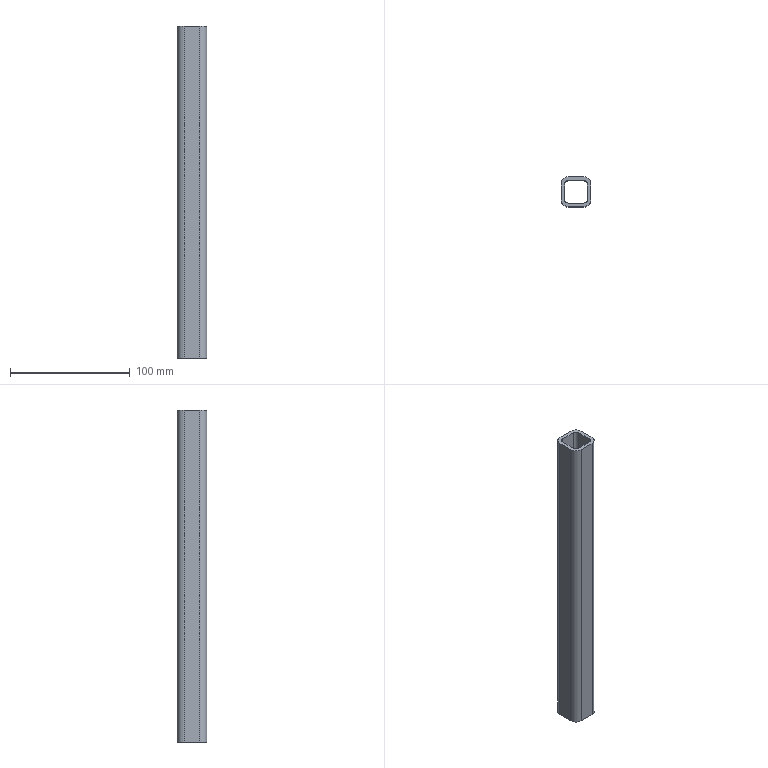Part | STEP file | ISO 10799-2 25x25x3 1784908143849 | 1 solid | 18 faces | box 25 x 25 x 277.531 mm | volume 66836 mm3 | plane 10 | cylinder 8 | commonest cylinder face diameters 6 x4 12 x4
STEP:
#1=CARTESIAN_POINT('',(-6.5,-9.5,290.031));
#2=VERTEX_POINT('',#1);
#3=CARTESIAN_POINT('',(6.5,-9.5,290.031));
#4=VERTEX_POINT('',#3);
#5=CARTESIAN_POINT('',(3.25,-9.5,290.031));
#6=DIRECTION('',(1.,0.,0.));
#7=VECTOR('',#6,10.);
#8=LINE('',#5,#7);
#9=EDGE_CURVE('',#2,#4,#8,.T.);
#10=ORIENTED_EDGE('',*,*,#9,.T.);
#11=CARTESIAN_POINT('',(6.5,-9.5,12.5));
#12=VERTEX_POINT('',#11);
#13=CARTESIAN_POINT('',(6.5,-9.5,0.));
#14=DIRECTION('',(0.,0.,1.));
#15=VECTOR('',#14,10.);
#16=LINE('',#13,#15);
#17=EDGE_CURVE('',#12,#4,#16,.T.);
#18=ORIENTED_EDGE('',*,*,#17,.F.);
#19=CARTESIAN_POINT('',(-6.5,-9.5,12.5));
#20=VERTEX_POINT('',#19);
#21=CARTESIAN_POINT('',(3.25,-9.5,12.5));
#22=DIRECTION('',(1.,0.,0.));
#23=VECTOR('',#22,10.);
#24=LINE('',#21,#23);
#25=EDGE_CURVE('',#20,#12,#24,.T.);
#26=ORIENTED_EDGE('',*,*,#25,.F.);
#27=CARTESIAN_POINT('',(-6.5,-9.5,0.));
#28=DIRECTION('',(0.,0.,1.));
#29=VECTOR('',#28,10.);
#30=LINE('',#27,#29);
#31=EDGE_CURVE('',#20,#2,#30,.T.);
#32=ORIENTED_EDGE('',*,*,#31,.T.);
#33=EDGE_LOOP('',(#10,#18,#26,#32));
#34=FACE_OUTER_BOUND('',#33,.T.);
#35=CARTESIAN_POINT('',(6.5,-9.5,0.));
#36=DIRECTION('',(0.,-1.,0.));
#37=DIRECTION('',(0.,0.,-1.));
#38=AXIS2_PLACEMENT_3D('',#35,#36,#37);
#39=PLANE('',#38);
#40=ADVANCED_FACE('',(#34),#39,.F.);
#41=CARTESIAN_POINT('',(9.5,-6.5,290.031));
#42=VERTEX_POINT('',#41);
#43=CARTESIAN_POINT('',(6.5,-6.5,290.031));
#44=DIRECTION('',(0.,0.,1.));
#45=DIRECTION('',(0.,1.,0.));
#46=AXIS2_PLACEMENT_3D('',#43,#44,#45);
#47=CIRCLE('',#46,3.);
#48=EDGE_CURVE('',#4,#42,#47,.T.);
#49=ORIENTED_EDGE('',*,*,#48,.T.);
#50=CARTESIAN_POINT('',(9.5,-6.5,12.5));
#51=VERTEX_POINT('',#50);
#52=CARTESIAN_POINT('',(9.5,-6.5,0.));
#53=DIRECTION('',(0.,0.,1.));
#54=VECTOR('',#53,10.);
#55=LINE('',#52,#54);
#56=EDGE_CURVE('',#51,#42,#55,.T.);
#57=ORIENTED_EDGE('',*,*,#56,.F.);
#58=CARTESIAN_POINT('',(6.5,-6.5,12.5));
#59=DIRECTION('',(0.,0.,1.));
#60=DIRECTION('',(0.,1.,0.));
#61=AXIS2_PLACEMENT_3D('',#58,#59,#60);
#62=CIRCLE('',#61,3.);
#63=EDGE_CURVE('',#12,#51,#62,.T.);
#64=ORIENTED_EDGE('',*,*,#63,.F.);
#65=ORIENTED_EDGE('',*,*,#17,.T.);
#66=EDGE_LOOP('',(#49,#57,#64,#65));
#67=FACE_OUTER_BOUND('',#66,.T.);
#68=CARTESIAN_POINT('',(6.5,-6.5,0.));
#69=DIRECTION('',(0.,0.,1.));
#70=DIRECTION('',(0.,1.,0.));
#71=AXIS2_PLACEMENT_3D('',#68,#69,#70);
#72=CYLINDRICAL_SURFACE('',#71,3.);
#73=ADVANCED_FACE('',(#67),#72,.F.);
#74=CARTESIAN_POINT('',(9.5,6.5,290.031));
#75=VERTEX_POINT('',#74);
#76=CARTESIAN_POINT('',(9.5,3.25,290.031));
#77=DIRECTION('',(0.,1.,0.));
#78=VECTOR('',#77,10.);
#79=LINE('',#76,#78);
#80=EDGE_CURVE('',#42,#75,#79,.T.);
#81=ORIENTED_EDGE('',*,*,#80,.T.);
#82=CARTESIAN_POINT('',(9.5,6.5,12.5));
#83=VERTEX_POINT('',#82);
#84=CARTESIAN_POINT('',(9.5,6.5,0.));
#85=DIRECTION('',(0.,0.,1.));
#86=VECTOR('',#85,10.);
#87=LINE('',#84,#86);
#88=EDGE_CURVE('',#83,#75,#87,.T.);
#89=ORIENTED_EDGE('',*,*,#88,.F.);
#90=CARTESIAN_POINT('',(9.5,3.25,12.5));
#91=DIRECTION('',(0.,1.,0.));
#92=VECTOR('',#91,10.);
#93=LINE('',#90,#92);
#94=EDGE_CURVE('',#51,#83,#93,.T.);
#95=ORIENTED_EDGE('',*,*,#94,.F.);
#96=ORIENTED_EDGE('',*,*,#56,.T.);
#97=EDGE_LOOP('',(#81,#89,#95,#96));
#98=FACE_OUTER_BOUND('',#97,.T.);
#99=CARTESIAN_POINT('',(9.5,6.5,0.));
#100=DIRECTION('',(1.,0.,0.));
#101=DIRECTION('',(0.,0.,-1.));
#102=AXIS2_PLACEMENT_3D('',#99,#100,#101);
#103=PLANE('',#102);
#104=ADVANCED_FACE('',(#98),#103,.F.);
#105=CARTESIAN_POINT('',(6.5,9.5,290.031));
#106=VERTEX_POINT('',#105);
#107=CARTESIAN_POINT('',(6.5,6.5,290.031));
#108=DIRECTION('',(0.,0.,1.));
#109=DIRECTION('',(-1.,0.,0.));
#110=AXIS2_PLACEMENT_3D('',#107,#108,#109);
#111=CIRCLE('',#110,3.);
#112=EDGE_CURVE('',#75,#106,#111,.T.);
#113=ORIENTED_EDGE('',*,*,#112,.T.);
#114=CARTESIAN_POINT('',(6.5,9.5,12.5));
#115=VERTEX_POINT('',#114);
#116=CARTESIAN_POINT('',(6.5,9.5,0.));
#117=DIRECTION('',(0.,0.,1.));
#118=VECTOR('',#117,10.);
#119=LINE('',#116,#118);
#120=EDGE_CURVE('',#115,#106,#119,.T.);
#121=ORIENTED_EDGE('',*,*,#120,.F.);
#122=CARTESIAN_POINT('',(6.5,6.5,12.5));
#123=DIRECTION('',(0.,0.,1.));
#124=DIRECTION('',(-1.,0.,0.));
#125=AXIS2_PLACEMENT_3D('',#122,#123,#124);
#126=CIRCLE('',#125,3.);
#127=EDGE_CURVE('',#83,#115,#126,.T.);
#128=ORIENTED_EDGE('',*,*,#127,.F.);
#129=ORIENTED_EDGE('',*,*,#88,.T.);
#130=EDGE_LOOP('',(#113,#121,#128,#129));
#131=FACE_OUTER_BOUND('',#130,.T.);
#132=CARTESIAN_POINT('',(6.5,6.5,0.));
#133=DIRECTION('',(0.,0.,1.));
#134=DIRECTION('',(-1.,0.,0.));
#135=AXIS2_PLACEMENT_3D('',#132,#133,#134);
#136=CYLINDRICAL_SURFACE('',#135,3.);
#137=ADVANCED_FACE('',(#131),#136,.F.);
#138=CARTESIAN_POINT('',(12.5,6.5,290.031));
#139=VERTEX_POINT('',#138);
#140=CARTESIAN_POINT('',(12.5,-6.5,290.031));
#141=VERTEX_POINT('',#140);
#142=CARTESIAN_POINT('',(12.5,3.25,290.031));
#143=DIRECTION('',(0.,-1.,0.));
#144=VECTOR('',#143,10.);
#145=LINE('',#142,#144);
#146=EDGE_CURVE('',#139,#141,#145,.T.);
#147=ORIENTED_EDGE('',*,*,#146,.T.);
#148=CARTESIAN_POINT('',(12.5,-6.5,12.5));
#149=VERTEX_POINT('',#148);
#150=CARTESIAN_POINT('',(12.5,-6.5,0.));
#151=DIRECTION('',(0.,0.,1.));
#152=VECTOR('',#151,10.);
#153=LINE('',#150,#152);
#154=EDGE_CURVE('',#149,#141,#153,.T.);
#155=ORIENTED_EDGE('',*,*,#154,.F.);
#156=CARTESIAN_POINT('',(12.5,6.5,12.5));
#157=VERTEX_POINT('',#156);
#158=CARTESIAN_POINT('',(12.5,3.25,12.5));
#159=DIRECTION('',(0.,-1.,0.));
#160=VECTOR('',#159,10.);
#161=LINE('',#158,#160);
#162=EDGE_CURVE('',#157,#149,#161,.T.);
#163=ORIENTED_EDGE('',*,*,#162,.F.);
#164=CARTESIAN_POINT('',(12.5,6.5,0.));
#165=DIRECTION('',(0.,0.,1.));
#166=VECTOR('',#165,10.);
#167=LINE('',#164,#166);
#168=EDGE_CURVE('',#157,#139,#167,.T.);
#169=ORIENTED_EDGE('',*,*,#168,.T.);
#170=EDGE_LOOP('',(#147,#155,#163,#169));
#171=FACE_OUTER_BOUND('',#170,.T.);
#172=CARTESIAN_POINT('',(12.5,6.5,0.));
#173=DIRECTION('',(1.,0.,0.));
#174=DIRECTION('',(0.,0.,-1.));
#175=AXIS2_PLACEMENT_3D('',#172,#173,#174);
#176=PLANE('',#175);
#177=ADVANCED_FACE('',(#171),#176,.T.);
#178=CARTESIAN_POINT('',(6.5,-12.5,290.031));
#179=VERTEX_POINT('',#178);
#180=CARTESIAN_POINT('',(6.5,-6.5,290.031));
#181=DIRECTION('',(0.,0.,-1.));
#182=DIRECTION('',(0.,1.,0.));
#183=AXIS2_PLACEMENT_3D('',#180,#181,#182);
#184=CIRCLE('',#183,6.);
#185=EDGE_CURVE('',#141,#179,#184,.T.);
#186=ORIENTED_EDGE('',*,*,#185,.T.);
#187=CARTESIAN_POINT('',(6.5,-12.5,12.5));
#188=VERTEX_POINT('',#187);
#189=CARTESIAN_POINT('',(6.5,-12.5,0.));
#190=DIRECTION('',(0.,0.,1.));
#191=VECTOR('',#190,10.);
#192=LINE('',#189,#191);
#193=EDGE_CURVE('',#188,#179,#192,.T.);
#194=ORIENTED_EDGE('',*,*,#193,.F.);
#195=CARTESIAN_POINT('',(6.5,-6.5,12.5));
#196=DIRECTION('',(0.,0.,-1.));
#197=DIRECTION('',(0.,1.,0.));
#198=AXIS2_PLACEMENT_3D('',#195,#196,#197);
#199=CIRCLE('',#198,6.);
#200=EDGE_CURVE('',#149,#188,#199,.T.);
#201=ORIENTED_EDGE('',*,*,#200,.F.);
#202=ORIENTED_EDGE('',*,*,#154,.T.);
#203=EDGE_LOOP('',(#186,#194,#201,#202));
#204=FACE_OUTER_BOUND('',#203,.T.);
#205=CARTESIAN_POINT('',(6.5,-6.5,0.));
#206=DIRECTION('',(0.,0.,1.));
#207=DIRECTION('',(0.,1.,0.));
#208=AXIS2_PLACEMENT_3D('',#205,#206,#207);
#209=CYLINDRICAL_SURFACE('',#208,6.);
#210=ADVANCED_FACE('',(#204),#209,.T.);
#211=CARTESIAN_POINT('',(-6.5,-12.5,290.031));
#212=VERTEX_POINT('',#211);
#213=CARTESIAN_POINT('',(3.25,-12.5,290.031));
#214=DIRECTION('',(-1.,0.,0.));
#215=VECTOR('',#214,10.);
#216=LINE('',#213,#215);
#217=EDGE_CURVE('',#179,#212,#216,.T.);
#218=ORIENTED_EDGE('',*,*,#217,.T.);
#219=CARTESIAN_POINT('',(-6.5,-12.5,12.5));
#220=VERTEX_POINT('',#219);
#221=CARTESIAN_POINT('',(-6.5,-12.5,0.));
#222=DIRECTION('',(0.,0.,1.));
#223=VECTOR('',#222,10.);
#224=LINE('',#221,#223);
#225=EDGE_CURVE('',#220,#212,#224,.T.);
#226=ORIENTED_EDGE('',*,*,#225,.F.);
#227=CARTESIAN_POINT('',(3.25,-12.5,12.5));
#228=DIRECTION('',(-1.,0.,0.));
#229=VECTOR('',#228,10.);
#230=LINE('',#227,#229);
#231=EDGE_CURVE('',#188,#220,#230,.T.);
#232=ORIENTED_EDGE('',*,*,#231,.F.);
#233=ORIENTED_EDGE('',*,*,#193,.T.);
#234=EDGE_LOOP('',(#218,#226,#232,#233));
#235=FACE_OUTER_BOUND('',#234,.T.);
#236=CARTESIAN_POINT('',(6.5,-12.5,0.));
#237=DIRECTION('',(0.,-1.,0.));
#238=DIRECTION('',(0.,0.,-1.));
#239=AXIS2_PLACEMENT_3D('',#236,#237,#238);
#240=PLANE('',#239);
#241=ADVANCED_FACE('',(#235),#240,.T.);
#242=CARTESIAN_POINT('',(-12.5,-6.5,290.031));
#243=VERTEX_POINT('',#242);
#244=CARTESIAN_POINT('',(-6.5,-6.5,290.031));
#245=DIRECTION('',(0.,0.,-1.));
#246=DIRECTION('',(1.,0.,0.));
#247=AXIS2_PLACEMENT_3D('',#244,#245,#246);
#248=CIRCLE('',#247,6.);
#249=EDGE_CURVE('',#212,#243,#248,.T.);
#250=ORIENTED_EDGE('',*,*,#249,.T.);
#251=CARTESIAN_POINT('',(-12.5,-6.5,12.5));
#252=VERTEX_POINT('',#251);
#253=CARTESIAN_POINT('',(-12.5,-6.5,0.));
#254=DIRECTION('',(0.,0.,1.));
#255=VECTOR('',#254,10.);
#256=LINE('',#253,#255);
#257=EDGE_CURVE('',#252,#243,#256,.T.);
#258=ORIENTED_EDGE('',*,*,#257,.F.);
#259=CARTESIAN_POINT('',(-6.5,-6.5,12.5));
#260=DIRECTION('',(0.,0.,-1.));
#261=DIRECTION('',(1.,0.,0.));
#262=AXIS2_PLACEMENT_3D('',#259,#260,#261);
#263=CIRCLE('',#262,6.);
#264=EDGE_CURVE('',#220,#252,#263,.T.);
#265=ORIENTED_EDGE('',*,*,#264,.F.);
#266=ORIENTED_EDGE('',*,*,#225,.T.);
#267=EDGE_LOOP('',(#250,#258,#265,#266));
#268=FACE_OUTER_BOUND('',#267,.T.);
#269=CARTESIAN_POINT('',(-6.5,-6.5,0.));
#270=DIRECTION('',(0.,0.,1.));
#271=DIRECTION('',(1.,0.,0.));
#272=AXIS2_PLACEMENT_3D('',#269,#270,#271);
#273=CYLINDRICAL_SURFACE('',#272,6.);
#274=ADVANCED_FACE('',(#268),#273,.T.);
#275=CARTESIAN_POINT('',(-6.5,9.5,290.031));
#276=VERTEX_POINT('',#275);
#277=CARTESIAN_POINT('',(-3.25,9.5,290.031));
#278=DIRECTION('',(-1.,0.,0.));
#279=VECTOR('',#278,10.);
#280=LINE('',#277,#279);
#281=EDGE_CURVE('',#106,#276,#280,.T.);
#282=ORIENTED_EDGE('',*,*,#281,.T.);
#283=CARTESIAN_POINT('',(-6.5,9.5,12.5));
#284=VERTEX_POINT('',#283);
#285=CARTESIAN_POINT('',(-6.5,9.5,0.));
#286=DIRECTION('',(0.,0.,1.));
#287=VECTOR('',#286,10.);
#288=LINE('',#285,#287);
#289=EDGE_CURVE('',#284,#276,#288,.T.);
#290=ORIENTED_EDGE('',*,*,#289,.F.);
#291=CARTESIAN_POINT('',(-3.25,9.5,12.5));
#292=DIRECTION('',(-1.,0.,0.));
#293=VECTOR('',#292,10.);
#294=LINE('',#291,#293);
#295=EDGE_CURVE('',#115,#284,#294,.T.);
#296=ORIENTED_EDGE('',*,*,#295,.F.);
#297=ORIENTED_EDGE('',*,*,#120,.T.);
#298=EDGE_LOOP('',(#282,#290,#296,#297));
#299=FACE_OUTER_BOUND('',#298,.T.);
#300=CARTESIAN_POINT('',(-6.5,9.5,0.));
#301=DIRECTION('',(0.,1.,0.));
#302=DIRECTION('',(0.,0.,1.));
#303=AXIS2_PLACEMENT_3D('',#300,#301,#302);
#304=PLANE('',#303);
#305=ADVANCED_FACE('',(#299),#304,.F.);
#306=CARTESIAN_POINT('',(-9.5,-6.5,290.031));
#307=VERTEX_POINT('',#306);
#308=CARTESIAN_POINT('',(-6.5,-6.5,290.031));
#309=DIRECTION('',(0.,0.,1.));
#310=DIRECTION('',(1.,0.,0.));
#311=AXIS2_PLACEMENT_3D('',#308,#309,#310);
#312=CIRCLE('',#311,3.);
#313=EDGE_CURVE('',#307,#2,#312,.T.);
#314=ORIENTED_EDGE('',*,*,#313,.T.);
#315=ORIENTED_EDGE('',*,*,#31,.F.);
#316=CARTESIAN_POINT('',(-9.5,-6.5,12.5));
#317=VERTEX_POINT('',#316);
#318=CARTESIAN_POINT('',(-6.5,-6.5,12.5));
#319=DIRECTION('',(0.,0.,1.));
#320=DIRECTION('',(1.,0.,0.));
#321=AXIS2_PLACEMENT_3D('',#318,#319,#320);
#322=CIRCLE('',#321,3.);
#323=EDGE_CURVE('',#317,#20,#322,.T.);
#324=ORIENTED_EDGE('',*,*,#323,.F.);
#325=CARTESIAN_POINT('',(-9.5,-6.5,0.));
#326=DIRECTION('',(0.,0.,1.));
#327=VECTOR('',#326,10.);
#328=LINE('',#325,#327);
#329=EDGE_CURVE('',#317,#307,#328,.T.);
#330=ORIENTED_EDGE('',*,*,#329,.T.);
#331=EDGE_LOOP('',(#314,#315,#324,#330));
#332=FACE_OUTER_BOUND('',#331,.T.);
#333=CARTESIAN_POINT('',(-6.5,-6.5,0.));
#334=DIRECTION('',(0.,0.,1.));
#335=DIRECTION('',(1.,0.,0.));
#336=AXIS2_PLACEMENT_3D('',#333,#334,#335);
#337=CYLINDRICAL_SURFACE('',#336,3.);
#338=ADVANCED_FACE('',(#332),#337,.F.);
#339=CARTESIAN_POINT('',(-9.5,6.5,290.031));
#340=VERTEX_POINT('',#339);
#341=CARTESIAN_POINT('',(-9.5,-3.25,290.031));
#342=DIRECTION('',(0.,-1.,0.));
#343=VECTOR('',#342,10.);
#344=LINE('',#341,#343);
#345=EDGE_CURVE('',#340,#307,#344,.T.);
#346=ORIENTED_EDGE('',*,*,#345,.T.);
#347=ORIENTED_EDGE('',*,*,#329,.F.);
#348=CARTESIAN_POINT('',(-9.5,6.5,12.5));
#349=VERTEX_POINT('',#348);
#350=CARTESIAN_POINT('',(-9.5,-3.25,12.5));
#351=DIRECTION('',(0.,-1.,0.));
#352=VECTOR('',#351,10.);
#353=LINE('',#350,#352);
#354=EDGE_CURVE('',#349,#317,#353,.T.);
#355=ORIENTED_EDGE('',*,*,#354,.F.);
#356=CARTESIAN_POINT('',(-9.5,6.5,0.));
#357=DIRECTION('',(0.,0.,1.));
#358=VECTOR('',#357,10.);
#359=LINE('',#356,#358);
#360=EDGE_CURVE('',#349,#340,#359,.T.);
#361=ORIENTED_EDGE('',*,*,#360,.T.);
#362=EDGE_LOOP('',(#346,#347,#355,#361));
#363=FACE_OUTER_BOUND('',#362,.T.);
#364=CARTESIAN_POINT('',(-9.5,-6.5,0.));
#365=DIRECTION('',(-1.,0.,0.));
#366=DIRECTION('',(0.,0.,1.));
#367=AXIS2_PLACEMENT_3D('',#364,#365,#366);
#368=PLANE('',#367);
#369=ADVANCED_FACE('',(#363),#368,.F.);
#370=CARTESIAN_POINT('',(-6.5,6.5,290.031));
#371=DIRECTION('',(0.,0.,1.));
#372=DIRECTION('',(0.,-1.,0.));
#373=AXIS2_PLACEMENT_3D('',#370,#371,#372);
#374=CIRCLE('',#373,3.);
#375=EDGE_CURVE('',#276,#340,#374,.T.);
#376=ORIENTED_EDGE('',*,*,#375,.T.);
#377=ORIENTED_EDGE('',*,*,#360,.F.);
#378=CARTESIAN_POINT('',(-6.5,6.5,12.5));
#379=DIRECTION('',(0.,0.,1.));
#380=DIRECTION('',(0.,-1.,0.));
#381=AXIS2_PLACEMENT_3D('',#378,#379,#380);
#382=CIRCLE('',#381,3.);
#383=EDGE_CURVE('',#284,#349,#382,.T.);
#384=ORIENTED_EDGE('',*,*,#383,.F.);
#385=ORIENTED_EDGE('',*,*,#289,.T.);
#386=EDGE_LOOP('',(#376,#377,#384,#385));
#387=FACE_OUTER_BOUND('',#386,.T.);
#388=CARTESIAN_POINT('',(-6.5,6.5,0.));
#389=DIRECTION('',(0.,0.,1.));
#390=DIRECTION('',(0.,-1.,0.));
#391=AXIS2_PLACEMENT_3D('',#388,#389,#390);
#392=CYLINDRICAL_SURFACE('',#391,3.);
#393=ADVANCED_FACE('',(#387),#392,.F.);
#394=CARTESIAN_POINT('',(-12.5,6.5,290.031));
#395=VERTEX_POINT('',#394);
#396=CARTESIAN_POINT('',(-12.5,-3.25,290.031));
#397=DIRECTION('',(0.,1.,0.));
#398=VECTOR('',#397,10.);
#399=LINE('',#396,#398);
#400=EDGE_CURVE('',#243,#395,#399,.T.);
#401=ORIENTED_EDGE('',*,*,#400,.T.);
#402=CARTESIAN_POINT('',(-12.5,6.5,12.5));
#403=VERTEX_POINT('',#402);
#404=CARTESIAN_POINT('',(-12.5,6.5,0.));
#405=DIRECTION('',(0.,0.,1.));
#406=VECTOR('',#405,10.);
#407=LINE('',#404,#406);
#408=EDGE_CURVE('',#403,#395,#407,.T.);
#409=ORIENTED_EDGE('',*,*,#408,.F.);
#410=CARTESIAN_POINT('',(-12.5,-3.25,12.5));
#411=DIRECTION('',(0.,1.,0.));
#412=VECTOR('',#411,10.);
#413=LINE('',#410,#412);
#414=EDGE_CURVE('',#252,#403,#413,.T.);
#415=ORIENTED_EDGE('',*,*,#414,.F.);
#416=ORIENTED_EDGE('',*,*,#257,.T.);
#417=EDGE_LOOP('',(#401,#409,#415,#416));
#418=FACE_OUTER_BOUND('',#417,.T.);
#419=CARTESIAN_POINT('',(-12.5,-6.5,0.));
#420=DIRECTION('',(-1.,0.,0.));
#421=DIRECTION('',(0.,0.,1.));
#422=AXIS2_PLACEMENT_3D('',#419,#420,#421);
#423=PLANE('',#422);
#424=ADVANCED_FACE('',(#418),#423,.T.);
#425=CARTESIAN_POINT('',(-6.5,12.5,290.031));
#426=VERTEX_POINT('',#425);
#427=CARTESIAN_POINT('',(-6.5,6.5,290.031));
#428=DIRECTION('',(0.,0.,-1.));
#429=DIRECTION('',(0.,-1.,0.));
#430=AXIS2_PLACEMENT_3D('',#427,#428,#429);
#431=CIRCLE('',#430,6.);
#432=EDGE_CURVE('',#395,#426,#431,.T.);
#433=ORIENTED_EDGE('',*,*,#432,.T.);
#434=CARTESIAN_POINT('',(-6.5,12.5,12.5));
#435=VERTEX_POINT('',#434);
#436=CARTESIAN_POINT('',(-6.5,12.5,0.));
#437=DIRECTION('',(0.,0.,1.));
#438=VECTOR('',#437,10.);
#439=LINE('',#436,#438);
#440=EDGE_CURVE('',#435,#426,#439,.T.);
#441=ORIENTED_EDGE('',*,*,#440,.F.);
#442=CARTESIAN_POINT('',(-6.5,6.5,12.5));
#443=DIRECTION('',(0.,0.,-1.));
#444=DIRECTION('',(0.,-1.,0.));
#445=AXIS2_PLACEMENT_3D('',#442,#443,#444);
#446=CIRCLE('',#445,6.);
#447=EDGE_CURVE('',#403,#435,#446,.T.);
#448=ORIENTED_EDGE('',*,*,#447,.F.);
#449=ORIENTED_EDGE('',*,*,#408,.T.);
#450=EDGE_LOOP('',(#433,#441,#448,#449));
#451=FACE_OUTER_BOUND('',#450,.T.);
#452=CARTESIAN_POINT('',(-6.5,6.5,0.));
#453=DIRECTION('',(0.,0.,1.));
#454=DIRECTION('',(0.,-1.,0.));
#455=AXIS2_PLACEMENT_3D('',#452,#453,#454);
#456=CYLINDRICAL_SURFACE('',#455,6.);
#457=ADVANCED_FACE('',(#451),#456,.T.);
#458=CARTESIAN_POINT('',(6.5,12.5,290.031));
#459=VERTEX_POINT('',#458);
#460=CARTESIAN_POINT('',(-3.25,12.5,290.031));
#461=DIRECTION('',(1.,0.,0.));
#462=VECTOR('',#461,10.);
#463=LINE('',#460,#462);
#464=EDGE_CURVE('',#426,#459,#463,.T.);
#465=ORIENTED_EDGE('',*,*,#464,.T.);
#466=CARTESIAN_POINT('',(6.5,12.5,12.5));
#467=VERTEX_POINT('',#466);
#468=CARTESIAN_POINT('',(6.5,12.5,0.));
#469=DIRECTION('',(0.,0.,1.));
#470=VECTOR('',#469,10.);
#471=LINE('',#468,#470);
#472=EDGE_CURVE('',#467,#459,#471,.T.);
#473=ORIENTED_EDGE('',*,*,#472,.F.);
#474=CARTESIAN_POINT('',(-3.25,12.5,12.5));
#475=DIRECTION('',(1.,0.,0.));
#476=VECTOR('',#475,10.);
#477=LINE('',#474,#476);
#478=EDGE_CURVE('',#435,#467,#477,.T.);
#479=ORIENTED_EDGE('',*,*,#478,.F.);
#480=ORIENTED_EDGE('',*,*,#440,.T.);
#481=EDGE_LOOP('',(#465,#473,#479,#480));
#482=FACE_OUTER_BOUND('',#481,.T.);
#483=CARTESIAN_POINT('',(-6.5,12.5,0.));
#484=DIRECTION('',(0.,1.,0.));
#485=DIRECTION('',(0.,0.,1.));
#486=AXIS2_PLACEMENT_3D('',#483,#484,#485);
#487=PLANE('',#486);
#488=ADVANCED_FACE('',(#482),#487,.T.);
#489=CARTESIAN_POINT('',(6.5,6.5,290.031));
#490=DIRECTION('',(0.,0.,-1.));
#491=DIRECTION('',(-1.,0.,0.));
#492=AXIS2_PLACEMENT_3D('',#489,#490,#491);
#493=CIRCLE('',#492,6.);
#494=EDGE_CURVE('',#459,#139,#493,.T.);
#495=ORIENTED_EDGE('',*,*,#494,.T.);
#496=ORIENTED_EDGE('',*,*,#168,.F.);
#497=CARTESIAN_POINT('',(6.5,6.5,12.5));
#498=DIRECTION('',(0.,0.,-1.));
#499=DIRECTION('',(-1.,0.,0.));
#500=AXIS2_PLACEMENT_3D('',#497,#498,#499);
#501=CIRCLE('',#500,6.);
#502=EDGE_CURVE('',#467,#157,#501,.T.);
#503=ORIENTED_EDGE('',*,*,#502,.F.);
#504=ORIENTED_EDGE('',*,*,#472,.T.);
#505=EDGE_LOOP('',(#495,#496,#503,#504));
#506=FACE_OUTER_BOUND('',#505,.T.);
#507=CARTESIAN_POINT('',(6.5,6.5,0.));
#508=DIRECTION('',(0.,0.,1.));
#509=DIRECTION('',(-1.,0.,0.));
#510=AXIS2_PLACEMENT_3D('',#507,#508,#509);
#511=CYLINDRICAL_SURFACE('',#510,6.);
#512=ADVANCED_FACE('',(#506),#511,.T.);
#513=ORIENTED_EDGE('',*,*,#414,.T.);
#514=ORIENTED_EDGE('',*,*,#447,.T.);
#515=ORIENTED_EDGE('',*,*,#478,.T.);
#516=ORIENTED_EDGE('',*,*,#502,.T.);
#517=ORIENTED_EDGE('',*,*,#162,.T.);
#518=ORIENTED_EDGE('',*,*,#200,.T.);
#519=ORIENTED_EDGE('',*,*,#231,.T.);
#520=ORIENTED_EDGE('',*,*,#264,.T.);
#521=EDGE_LOOP('',(#513,#514,#515,#516,#517,#518,#519,#520));
#522=FACE_OUTER_BOUND('',#521,.T.);
#523=ORIENTED_EDGE('',*,*,#295,.T.);
#524=ORIENTED_EDGE('',*,*,#383,.T.);
#525=ORIENTED_EDGE('',*,*,#354,.T.);
#526=ORIENTED_EDGE('',*,*,#323,.T.);
#527=ORIENTED_EDGE('',*,*,#25,.T.);
#528=ORIENTED_EDGE('',*,*,#63,.T.);
#529=ORIENTED_EDGE('',*,*,#94,.T.);
#530=ORIENTED_EDGE('',*,*,#127,.T.);
#531=EDGE_LOOP('',(#523,#524,#525,#526,#527,#528,#529,#530));
#532=FACE_BOUND('',#531,.T.);
#533=CARTESIAN_POINT('',(0.,0.,12.5));
#534=DIRECTION('',(0.,0.,1.));
#535=DIRECTION('',(1.,0.,0.));
#536=AXIS2_PLACEMENT_3D('',#533,#534,#535);
#537=PLANE('',#536);
#538=ADVANCED_FACE('',(#522,#532),#537,.F.);
#539=ORIENTED_EDGE('',*,*,#400,.F.);
#540=ORIENTED_EDGE('',*,*,#249,.F.);
#541=ORIENTED_EDGE('',*,*,#217,.F.);
#542=ORIENTED_EDGE('',*,*,#185,.F.);
#543=ORIENTED_EDGE('',*,*,#146,.F.);
#544=ORIENTED_EDGE('',*,*,#494,.F.);
#545=ORIENTED_EDGE('',*,*,#464,.F.);
#546=ORIENTED_EDGE('',*,*,#432,.F.);
#547=EDGE_LOOP('',(#539,#540,#541,#542,#543,#544,#545,#546));
#548=FACE_OUTER_BOUND('',#547,.T.);
#549=ORIENTED_EDGE('',*,*,#281,.F.);
#550=ORIENTED_EDGE('',*,*,#112,.F.);
#551=ORIENTED_EDGE('',*,*,#80,.F.);
#552=ORIENTED_EDGE('',*,*,#48,.F.);
#553=ORIENTED_EDGE('',*,*,#9,.F.);
#554=ORIENTED_EDGE('',*,*,#313,.F.);
#555=ORIENTED_EDGE('',*,*,#345,.F.);
#556=ORIENTED_EDGE('',*,*,#375,.F.);
#557=EDGE_LOOP('',(#549,#550,#551,#552,#553,#554,#555,#556));
#558=FACE_BOUND('',#557,.T.);
#559=CARTESIAN_POINT('',(0.,0.,290.031));
#560=DIRECTION('',(0.,0.,1.));
#561=DIRECTION('',(1.,0.,0.));
#562=AXIS2_PLACEMENT_3D('',#559,#560,#561);
#563=PLANE('',#562);
#564=ADVANCED_FACE('',(#548,#558),#563,.T.);
#565=CLOSED_SHELL('',(#40,#73,#104,#137,#177,#210,#241,#274,#305,#338,#369,#393,#424,#457,#488,#512,#538,#564));
#566=MANIFOLD_SOLID_BREP('',#565);
#567=(LENGTH_UNIT()NAMED_UNIT(*)SI_UNIT(.MILLI.,.METRE.));
#568=UNCERTAINTY_MEASURE_WITH_UNIT(LENGTH_MEASURE(0.01),#567,'','');
#569=(NAMED_UNIT(*)PLANE_ANGLE_UNIT()SI_UNIT($,.RADIAN.));
#570=(NAMED_UNIT(*)SI_UNIT($,.STERADIAN.)SOLID_ANGLE_UNIT());
#571=(GEOMETRIC_REPRESENTATION_CONTEXT(3)GLOBAL_UNCERTAINTY_ASSIGNED_CONTEXT((#568))GLOBAL_UNIT_ASSIGNED_CONTEXT((#567,#569,#570))REPRESENTATION_CONTEXT('',''));
#572=ADVANCED_BREP_SHAPE_REPRESENTATION('',(#566),#571);